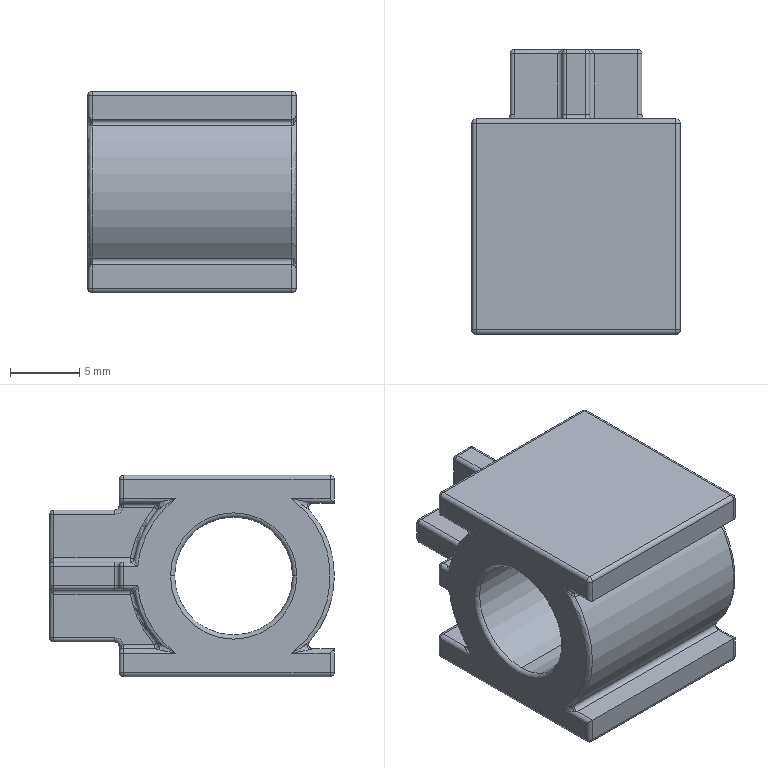Part | SolidWorks | features BaseBody 1 | 1 solid | 197 faces | box 15 x 20.5 x 14.5 mm | volume 2375 mm3 | cylinder 88 | plane 29 | sphere 29 | spline 29 | torus 22 | commonest cylinder face diameters 0.6 x81 14.5 x5 8.5 x2